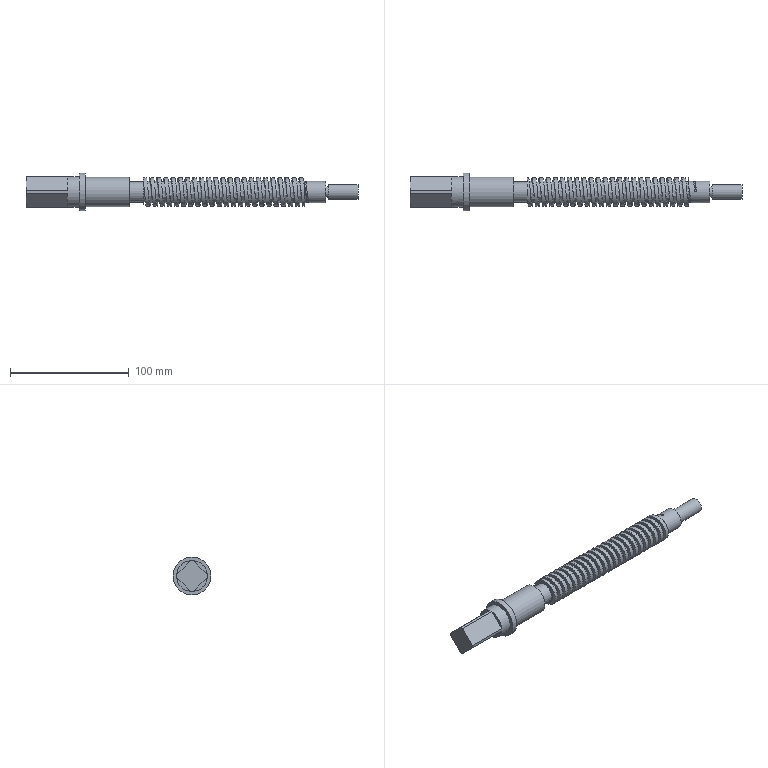Part | NX | features CYLINDER 6, DATUM_CSYS 2, RECT_GROOVE 2, SKETCH 2, DATUM_ON_PATH 1, EXTRUDE 1, HELIX 1, SKIN 1, SUBTRACT 1, SYMBOLIC_THREAD 1 | 1 solid | 32 faces | box 280 x 32 x 32 mm | volume 99870 mm3 | plane 17 | cylinder 10 | spline 5 | commonest cylinder face diameters 18 x3 9 x1 12.423 x1 17 x1 23.8 x1 25 x1